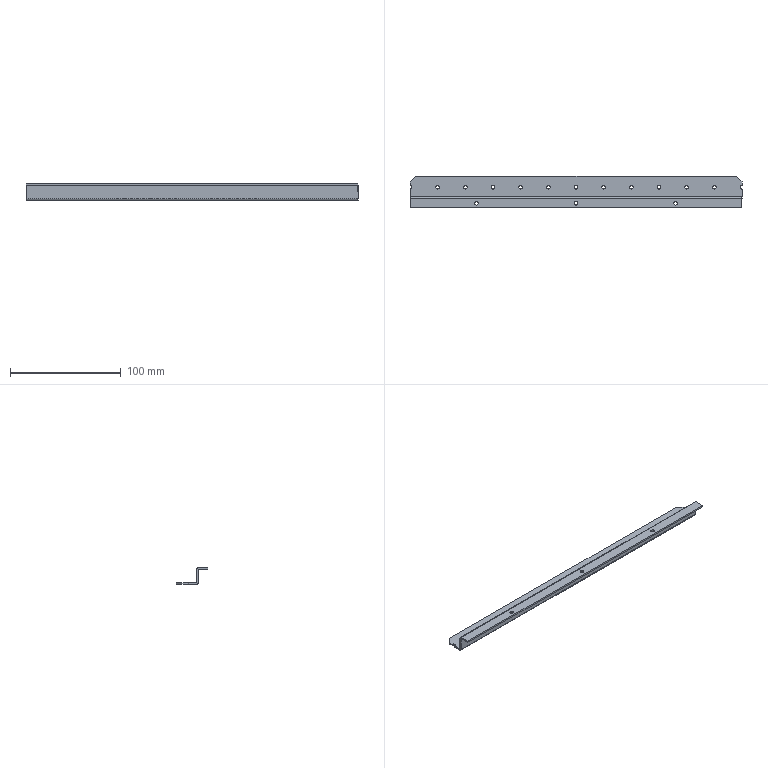Part | SolidWorks | features LPattern 4, EdgeFlange 2, ICE 2, Chamfer 1, FlatPattern 1, SMBaseFlange 1, SheetMetal 1 | 1 solid | 57 faces | box 300 x 28.5 x 15 mm | volume 18353 mm3 | cylinder 35 | plane 22 | commonest cylinder face diameters 3.2 x33 0.2 x2